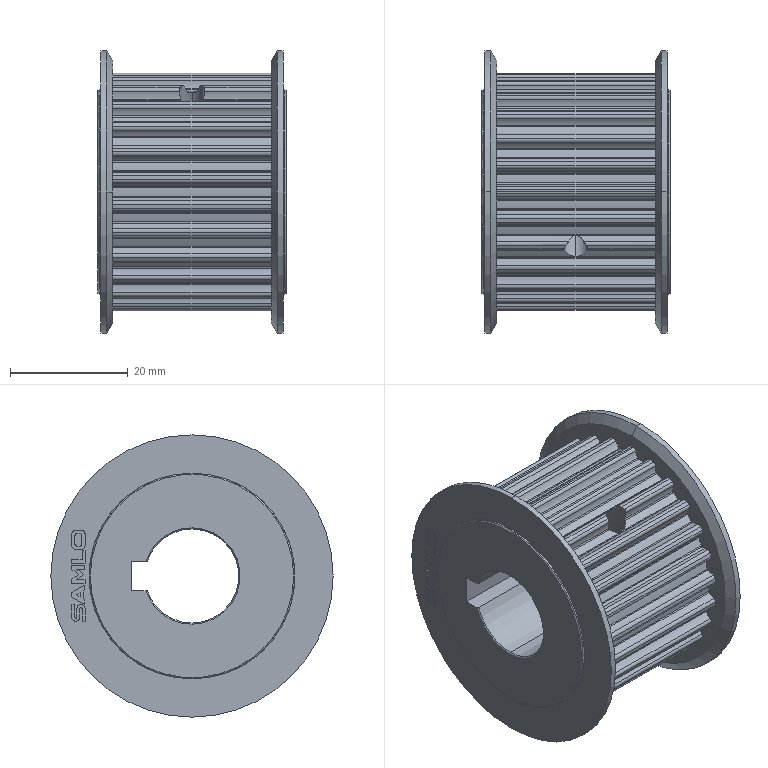Part | SolidWorks | features BaseBody 1 | 1 solid | 343 faces | box 32 x 48 x 48 mm | volume 32144 mm3 | cylinder 268 | plane 61 | cone 14 | commonest cylinder face diameters 1.1 x64 0.5 x63 6.55 x57 40.42 x28 36.88 x27 0.523 x4